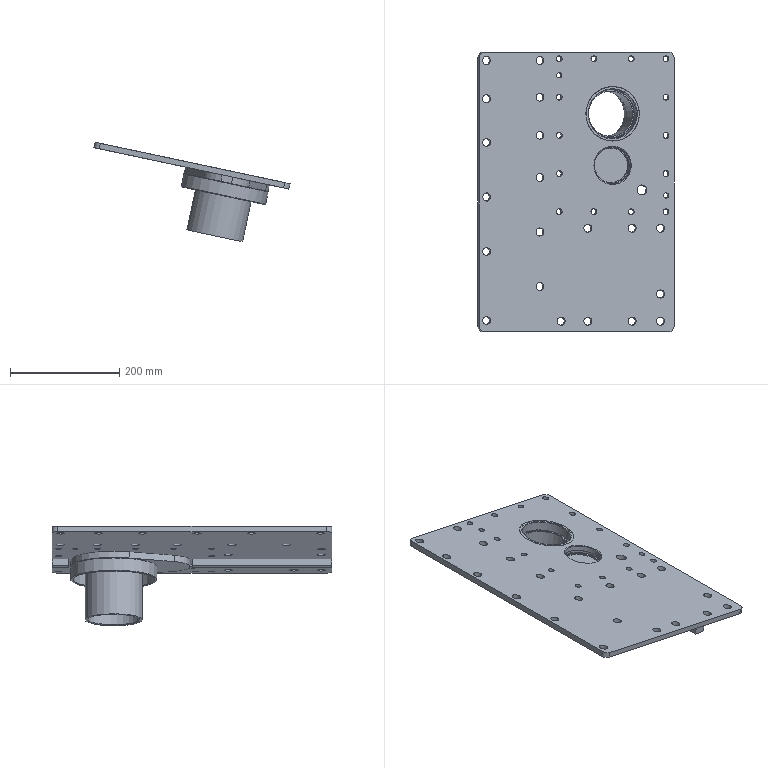Part | STEP file | HL4GZ-1.862.061 (gearbox cover) | 8 solids | 113 faces | box 359.103 x 512.5 x 182.227 mm | volume 2369356 mm3 | cylinder 57 | plane 45 | cone 8 | torus 3 | commonest cylinder face diameters 15 x20 11 x14 20 x4 90 x3 10 x2 68 x2